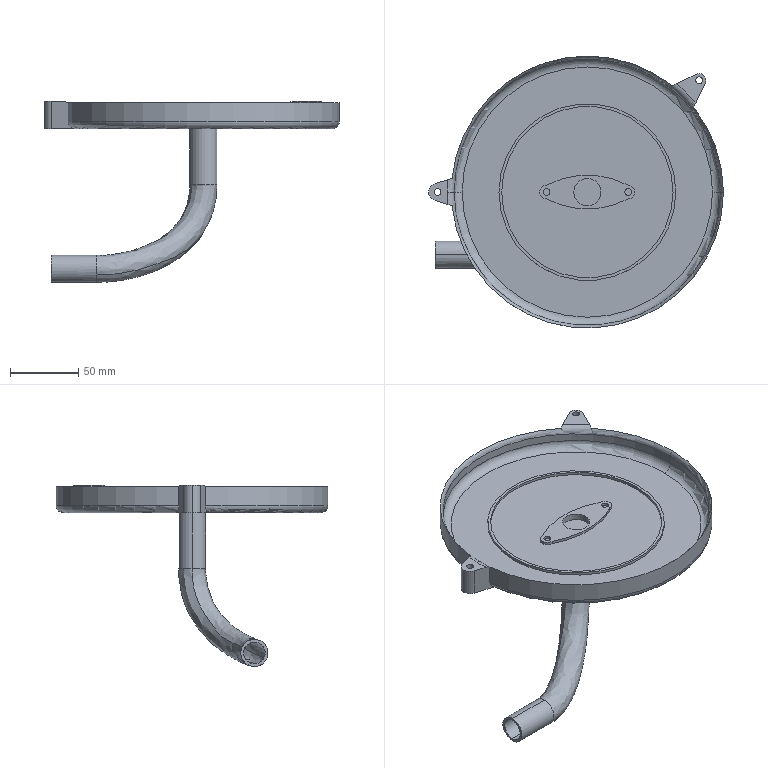Part | SolidWorks | features ICE 6, 3DProfileFeature 2, Fillet 2, Extrusion 1, Shell 1, Sweep 1 | 2 solids | 61 faces | box 216.698 x 200 x 133.163 mm | volume 149560 mm3 | cylinder 34 | plane 16 | torus 7 | spline 4 | commonest cylinder face diameters 5 x8 20 x6 16 x4 10 x3 13.142 x2 126 x2